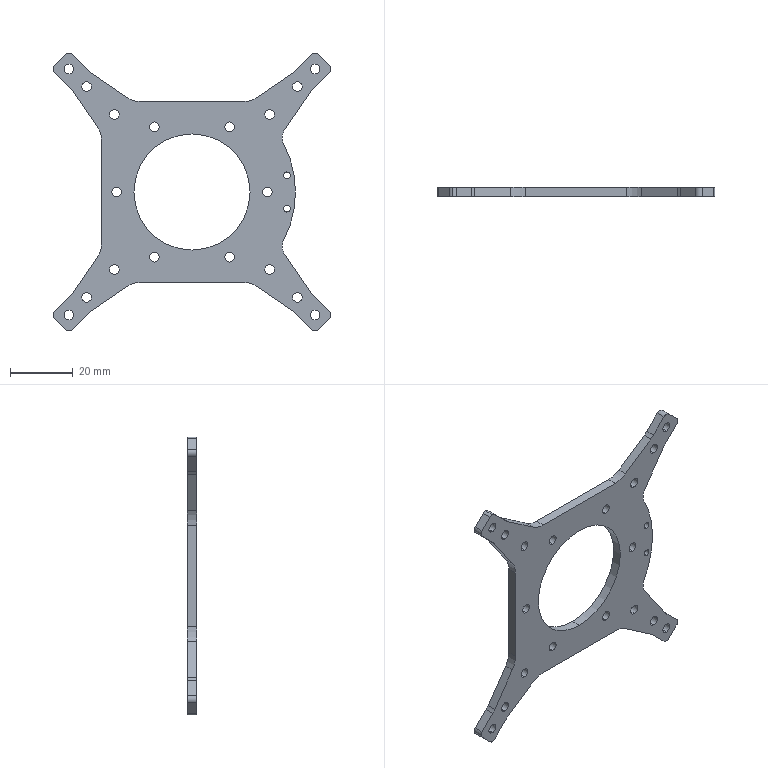Part | SolidWorks | features Fillet 3, Extrusion 1, ICE 1 | 1 solid | 98 faces | box 88.56 x 3 x 88.56 mm | volume 9081 mm3 | cylinder 71 | plane 27 | commonest cylinder face diameters 3.1 x36 16 x14 3 x10 2.1 x4 6 x4 37 x2